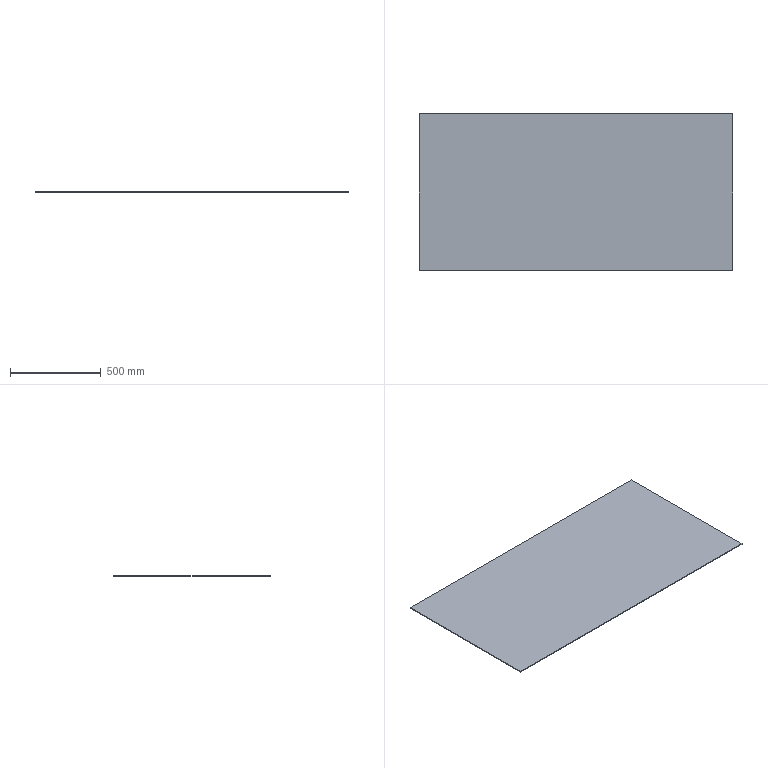Part | STEP file | 粉仓楼梯通道花纹Plate | 1 solid | 6 faces | box 1721 x 860 x 4 mm | volume 5920240 mm3 | plane 6
STEP:
#1=CARTESIAN_POINT('',(0.,0.,0.));
#2=DIRECTION('',(0.,0.,1.));
#3=DIRECTION('',(1.,0.,0.));
#4=AXIS2_PLACEMENT_3D('',#1,#2,#3);
#5=CARTESIAN_POINT('',(1588.,-50.,0.));
#6=VERTEX_POINT('',#5);
#7=CARTESIAN_POINT('',(1588.,810.,0.));
#8=VERTEX_POINT('',#7);
#9=CARTESIAN_POINT('',(1588.,810.,0.));
#10=DIRECTION('',(0.,1.,0.));
#11=VECTOR('',#10,1.);
#12=LINE('',#9,#11);
#13=CARTESIAN_POINT('',(1588.,810.,4.));
#14=DIRECTION('',(-1.,0.,0.));
#15=DIRECTION('',(0.,-1.,0.));
#16=AXIS2_PLACEMENT_3D('',#13,#14,#15);
#17=PLANE('',#16);
#18=CARTESIAN_POINT('',(0.,-4.));
#19=DIRECTION('',(-1.,0.));
#20=VECTOR('',#19,1.);
#21=LINE('',#18,#20);
#22=(GEOMETRIC_REPRESENTATION_CONTEXT(2)PARAMETRIC_REPRESENTATION_CONTEXT()REPRESENTATION_CONTEXT('',''));
#23=DEFINITIONAL_REPRESENTATION('',(#21),#22);
#24=PCURVE('',#17,#23);
#25=CARTESIAN_POINT('',(0.,0.,0.));
#26=DIRECTION('',(0.,0.,1.));
#27=DIRECTION('',(1.,0.,0.));
#28=AXIS2_PLACEMENT_3D('',#25,#26,#27);
#29=PLANE('',#28);
#30=CARTESIAN_POINT('',(1588.,810.));
#31=DIRECTION('',(0.,1.));
#32=VECTOR('',#31,1.);
#33=LINE('',#30,#32);
#34=(GEOMETRIC_REPRESENTATION_CONTEXT(2)PARAMETRIC_REPRESENTATION_CONTEXT()REPRESENTATION_CONTEXT('',''));
#35=DEFINITIONAL_REPRESENTATION('',(#33),#34);
#36=PCURVE('',#29,#35);
#37=SURFACE_CURVE('',#12,(#24,#36),.PCURVE_S1.);
#38=EDGE_CURVE('',#6,#8,#37,.T.);
#39=ORIENTED_EDGE('',*,*,#38,.T.);
#40=CARTESIAN_POINT('',(1588.,810.,4.));
#41=VERTEX_POINT('',#40);
#42=CARTESIAN_POINT('',(1588.,810.,4.));
#43=DIRECTION('',(0.,0.,-1.));
#44=VECTOR('',#43,1.);
#45=LINE('',#42,#44);
#46=CARTESIAN_POINT('',(0.,0.));
#47=DIRECTION('',(0.,-1.));
#48=VECTOR('',#47,1.);
#49=LINE('',#46,#48);
#50=(GEOMETRIC_REPRESENTATION_CONTEXT(2)PARAMETRIC_REPRESENTATION_CONTEXT()REPRESENTATION_CONTEXT('',''));
#51=DEFINITIONAL_REPRESENTATION('',(#49),#50);
#52=PCURVE('',#17,#51);
#53=CARTESIAN_POINT('',(-133.,810.,4.));
#54=DIRECTION('',(0.,-1.,0.));
#55=DIRECTION('',(1.,0.,0.));
#56=AXIS2_PLACEMENT_3D('',#53,#54,#55);
#57=PLANE('',#56);
#58=CARTESIAN_POINT('',(1721.,0.));
#59=DIRECTION('',(0.,-1.));
#60=VECTOR('',#59,1.);
#61=LINE('',#58,#60);
#62=(GEOMETRIC_REPRESENTATION_CONTEXT(2)PARAMETRIC_REPRESENTATION_CONTEXT()REPRESENTATION_CONTEXT('',''));
#63=DEFINITIONAL_REPRESENTATION('',(#61),#62);
#64=PCURVE('',#57,#63);
#65=SURFACE_CURVE('',#45,(#52,#64),.PCURVE_S1.);
#66=EDGE_CURVE('',#41,#8,#65,.T.);
#67=ORIENTED_EDGE('',*,*,#66,.F.);
#68=CARTESIAN_POINT('',(1588.,-50.,4.));
#69=VERTEX_POINT('',#68);
#70=CARTESIAN_POINT('',(1588.,810.,4.));
#71=DIRECTION('',(0.,1.,0.));
#72=VECTOR('',#71,1.);
#73=LINE('',#70,#72);
#74=CARTESIAN_POINT('',(0.,0.));
#75=DIRECTION('',(-1.,0.));
#76=VECTOR('',#75,1.);
#77=LINE('',#74,#76);
#78=(GEOMETRIC_REPRESENTATION_CONTEXT(2)PARAMETRIC_REPRESENTATION_CONTEXT()REPRESENTATION_CONTEXT('',''));
#79=DEFINITIONAL_REPRESENTATION('',(#77),#78);
#80=PCURVE('',#17,#79);
#81=CARTESIAN_POINT('',(0.,0.,4.));
#82=DIRECTION('',(0.,0.,1.));
#83=DIRECTION('',(1.,0.,0.));
#84=AXIS2_PLACEMENT_3D('',#81,#82,#83);
#85=PLANE('',#84);
#86=CARTESIAN_POINT('',(1588.,810.));
#87=DIRECTION('',(0.,1.));
#88=VECTOR('',#87,1.);
#89=LINE('',#86,#88);
#90=(GEOMETRIC_REPRESENTATION_CONTEXT(2)PARAMETRIC_REPRESENTATION_CONTEXT()REPRESENTATION_CONTEXT('',''));
#91=DEFINITIONAL_REPRESENTATION('',(#89),#90);
#92=PCURVE('',#85,#91);
#93=SURFACE_CURVE('',#73,(#80,#92),.PCURVE_S1.);
#94=EDGE_CURVE('',#69,#41,#93,.T.);
#95=ORIENTED_EDGE('',*,*,#94,.F.);
#96=CARTESIAN_POINT('',(1588.,-50.,4.));
#97=DIRECTION('',(0.,0.,-1.));
#98=VECTOR('',#97,1.);
#99=LINE('',#96,#98);
#100=CARTESIAN_POINT('',(860.,0.));
#101=DIRECTION('',(0.,-1.));
#102=VECTOR('',#101,1.);
#103=LINE('',#100,#102);
#104=(GEOMETRIC_REPRESENTATION_CONTEXT(2)PARAMETRIC_REPRESENTATION_CONTEXT()REPRESENTATION_CONTEXT('',''));
#105=DEFINITIONAL_REPRESENTATION('',(#103),#104);
#106=PCURVE('',#17,#105);
#107=CARTESIAN_POINT('',(-133.,-50.,4.));
#108=DIRECTION('',(0.,1.,0.));
#109=DIRECTION('',(-1.,0.,0.));
#110=AXIS2_PLACEMENT_3D('',#107,#108,#109);
#111=PLANE('',#110);
#112=CARTESIAN_POINT('',(-1721.,0.));
#113=DIRECTION('',(0.,-1.));
#114=VECTOR('',#113,1.);
#115=LINE('',#112,#114);
#116=(GEOMETRIC_REPRESENTATION_CONTEXT(2)PARAMETRIC_REPRESENTATION_CONTEXT()REPRESENTATION_CONTEXT('',''));
#117=DEFINITIONAL_REPRESENTATION('',(#115),#116);
#118=PCURVE('',#111,#117);
#119=SURFACE_CURVE('',#99,(#106,#118),.PCURVE_S1.);
#120=EDGE_CURVE('',#69,#6,#119,.T.);
#121=ORIENTED_EDGE('',*,*,#120,.T.);
#122=EDGE_LOOP('',(#39,#67,#95,#121));
#123=FACE_BOUND('',#122,.T.);
#124=ADVANCED_FACE('',(#123),#17,.F.);
#125=CARTESIAN_POINT('',(-133.,810.,0.));
#126=VERTEX_POINT('',#125);
#127=CARTESIAN_POINT('',(-133.,810.,0.));
#128=DIRECTION('',(-1.,0.,0.));
#129=VECTOR('',#128,1.);
#130=LINE('',#127,#129);
#131=CARTESIAN_POINT('',(0.,-4.));
#132=DIRECTION('',(-1.,0.));
#133=VECTOR('',#132,1.);
#134=LINE('',#131,#133);
#135=(GEOMETRIC_REPRESENTATION_CONTEXT(2)PARAMETRIC_REPRESENTATION_CONTEXT()REPRESENTATION_CONTEXT('',''));
#136=DEFINITIONAL_REPRESENTATION('',(#134),#135);
#137=PCURVE('',#57,#136);
#138=CARTESIAN_POINT('',(-133.,810.));
#139=DIRECTION('',(-1.,0.));
#140=VECTOR('',#139,1.);
#141=LINE('',#138,#140);
#142=(GEOMETRIC_REPRESENTATION_CONTEXT(2)PARAMETRIC_REPRESENTATION_CONTEXT()REPRESENTATION_CONTEXT('',''));
#143=DEFINITIONAL_REPRESENTATION('',(#141),#142);
#144=PCURVE('',#29,#143);
#145=SURFACE_CURVE('',#130,(#137,#144),.PCURVE_S1.);
#146=EDGE_CURVE('',#8,#126,#145,.T.);
#147=ORIENTED_EDGE('',*,*,#146,.T.);
#148=CARTESIAN_POINT('',(-133.,810.,4.));
#149=VERTEX_POINT('',#148);
#150=CARTESIAN_POINT('',(-133.,810.,4.));
#151=DIRECTION('',(0.,0.,-1.));
#152=VECTOR('',#151,1.);
#153=LINE('',#150,#152);
#154=CARTESIAN_POINT('',(0.,0.));
#155=DIRECTION('',(0.,-1.));
#156=VECTOR('',#155,1.);
#157=LINE('',#154,#156);
#158=(GEOMETRIC_REPRESENTATION_CONTEXT(2)PARAMETRIC_REPRESENTATION_CONTEXT()REPRESENTATION_CONTEXT('',''));
#159=DEFINITIONAL_REPRESENTATION('',(#157),#158);
#160=PCURVE('',#57,#159);
#161=CARTESIAN_POINT('',(-133.,810.,4.));
#162=DIRECTION('',(1.,0.,0.));
#163=DIRECTION('',(0.,1.,0.));
#164=AXIS2_PLACEMENT_3D('',#161,#162,#163);
#165=PLANE('',#164);
#166=CARTESIAN_POINT('',(0.,0.));
#167=DIRECTION('',(0.,-1.));
#168=VECTOR('',#167,1.);
#169=LINE('',#166,#168);
#170=(GEOMETRIC_REPRESENTATION_CONTEXT(2)PARAMETRIC_REPRESENTATION_CONTEXT()REPRESENTATION_CONTEXT('',''));
#171=DEFINITIONAL_REPRESENTATION('',(#169),#170);
#172=PCURVE('',#165,#171);
#173=SURFACE_CURVE('',#153,(#160,#172),.PCURVE_S1.);
#174=EDGE_CURVE('',#149,#126,#173,.T.);
#175=ORIENTED_EDGE('',*,*,#174,.F.);
#176=CARTESIAN_POINT('',(-133.,810.,4.));
#177=DIRECTION('',(-1.,0.,0.));
#178=VECTOR('',#177,1.);
#179=LINE('',#176,#178);
#180=CARTESIAN_POINT('',(0.,0.));
#181=DIRECTION('',(-1.,0.));
#182=VECTOR('',#181,1.);
#183=LINE('',#180,#182);
#184=(GEOMETRIC_REPRESENTATION_CONTEXT(2)PARAMETRIC_REPRESENTATION_CONTEXT()REPRESENTATION_CONTEXT('',''));
#185=DEFINITIONAL_REPRESENTATION('',(#183),#184);
#186=PCURVE('',#57,#185);
#187=CARTESIAN_POINT('',(-133.,810.));
#188=DIRECTION('',(-1.,0.));
#189=VECTOR('',#188,1.);
#190=LINE('',#187,#189);
#191=(GEOMETRIC_REPRESENTATION_CONTEXT(2)PARAMETRIC_REPRESENTATION_CONTEXT()REPRESENTATION_CONTEXT('',''));
#192=DEFINITIONAL_REPRESENTATION('',(#190),#191);
#193=PCURVE('',#85,#192);
#194=SURFACE_CURVE('',#179,(#186,#193),.PCURVE_S1.);
#195=EDGE_CURVE('',#41,#149,#194,.T.);
#196=ORIENTED_EDGE('',*,*,#195,.F.);
#197=ORIENTED_EDGE('',*,*,#66,.T.);
#198=EDGE_LOOP('',(#147,#175,#196,#197));
#199=FACE_BOUND('',#198,.T.);
#200=ADVANCED_FACE('',(#199),#57,.F.);
#201=CARTESIAN_POINT('',(-133.,-50.,0.));
#202=VERTEX_POINT('',#201);
#203=CARTESIAN_POINT('',(-133.,810.,0.));
#204=DIRECTION('',(0.,-1.,0.));
#205=VECTOR('',#204,1.);
#206=LINE('',#203,#205);
#207=CARTESIAN_POINT('',(0.,-4.));
#208=DIRECTION('',(-1.,0.));
#209=VECTOR('',#208,1.);
#210=LINE('',#207,#209);
#211=(GEOMETRIC_REPRESENTATION_CONTEXT(2)PARAMETRIC_REPRESENTATION_CONTEXT()REPRESENTATION_CONTEXT('',''));
#212=DEFINITIONAL_REPRESENTATION('',(#210),#211);
#213=PCURVE('',#165,#212);
#214=CARTESIAN_POINT('',(-133.,810.));
#215=DIRECTION('',(0.,-1.));
#216=VECTOR('',#215,1.);
#217=LINE('',#214,#216);
#218=(GEOMETRIC_REPRESENTATION_CONTEXT(2)PARAMETRIC_REPRESENTATION_CONTEXT()REPRESENTATION_CONTEXT('',''));
#219=DEFINITIONAL_REPRESENTATION('',(#217),#218);
#220=PCURVE('',#29,#219);
#221=SURFACE_CURVE('',#206,(#213,#220),.PCURVE_S1.);
#222=EDGE_CURVE('',#126,#202,#221,.T.);
#223=ORIENTED_EDGE('',*,*,#222,.T.);
#224=CARTESIAN_POINT('',(-133.,-50.,4.));
#225=VERTEX_POINT('',#224);
#226=CARTESIAN_POINT('',(-133.,-50.,4.));
#227=DIRECTION('',(0.,0.,-1.));
#228=VECTOR('',#227,1.);
#229=LINE('',#226,#228);
#230=CARTESIAN_POINT('',(-860.,0.));
#231=DIRECTION('',(0.,-1.));
#232=VECTOR('',#231,1.);
#233=LINE('',#230,#232);
#234=(GEOMETRIC_REPRESENTATION_CONTEXT(2)PARAMETRIC_REPRESENTATION_CONTEXT()REPRESENTATION_CONTEXT('',''));
#235=DEFINITIONAL_REPRESENTATION('',(#233),#234);
#236=PCURVE('',#165,#235);
#237=CARTESIAN_POINT('',(0.,0.));
#238=DIRECTION('',(0.,-1.));
#239=VECTOR('',#238,1.);
#240=LINE('',#237,#239);
#241=(GEOMETRIC_REPRESENTATION_CONTEXT(2)PARAMETRIC_REPRESENTATION_CONTEXT()REPRESENTATION_CONTEXT('',''));
#242=DEFINITIONAL_REPRESENTATION('',(#240),#241);
#243=PCURVE('',#111,#242);
#244=SURFACE_CURVE('',#229,(#236,#243),.PCURVE_S1.);
#245=EDGE_CURVE('',#225,#202,#244,.T.);
#246=ORIENTED_EDGE('',*,*,#245,.F.);
#247=CARTESIAN_POINT('',(-133.,810.,4.));
#248=DIRECTION('',(0.,-1.,0.));
#249=VECTOR('',#248,1.);
#250=LINE('',#247,#249);
#251=CARTESIAN_POINT('',(0.,0.));
#252=DIRECTION('',(-1.,0.));
#253=VECTOR('',#252,1.);
#254=LINE('',#251,#253);
#255=(GEOMETRIC_REPRESENTATION_CONTEXT(2)PARAMETRIC_REPRESENTATION_CONTEXT()REPRESENTATION_CONTEXT('',''));
#256=DEFINITIONAL_REPRESENTATION('',(#254),#255);
#257=PCURVE('',#165,#256);
#258=CARTESIAN_POINT('',(-133.,810.));
#259=DIRECTION('',(0.,-1.));
#260=VECTOR('',#259,1.);
#261=LINE('',#258,#260);
#262=(GEOMETRIC_REPRESENTATION_CONTEXT(2)PARAMETRIC_REPRESENTATION_CONTEXT()REPRESENTATION_CONTEXT('',''));
#263=DEFINITIONAL_REPRESENTATION('',(#261),#262);
#264=PCURVE('',#85,#263);
#265=SURFACE_CURVE('',#250,(#257,#264),.PCURVE_S1.);
#266=EDGE_CURVE('',#149,#225,#265,.T.);
#267=ORIENTED_EDGE('',*,*,#266,.F.);
#268=ORIENTED_EDGE('',*,*,#174,.T.);
#269=EDGE_LOOP('',(#223,#246,#267,#268));
#270=FACE_BOUND('',#269,.T.);
#271=ADVANCED_FACE('',(#270),#165,.F.);
#272=CARTESIAN_POINT('',(-133.,-50.,0.));
#273=DIRECTION('',(1.,0.,0.));
#274=VECTOR('',#273,1.);
#275=LINE('',#272,#274);
#276=CARTESIAN_POINT('',(0.,-4.));
#277=DIRECTION('',(-1.,0.));
#278=VECTOR('',#277,1.);
#279=LINE('',#276,#278);
#280=(GEOMETRIC_REPRESENTATION_CONTEXT(2)PARAMETRIC_REPRESENTATION_CONTEXT()REPRESENTATION_CONTEXT('',''));
#281=DEFINITIONAL_REPRESENTATION('',(#279),#280);
#282=PCURVE('',#111,#281);
#283=CARTESIAN_POINT('',(-133.,-50.));
#284=DIRECTION('',(1.,0.));
#285=VECTOR('',#284,1.);
#286=LINE('',#283,#285);
#287=(GEOMETRIC_REPRESENTATION_CONTEXT(2)PARAMETRIC_REPRESENTATION_CONTEXT()REPRESENTATION_CONTEXT('',''));
#288=DEFINITIONAL_REPRESENTATION('',(#286),#287);
#289=PCURVE('',#29,#288);
#290=SURFACE_CURVE('',#275,(#282,#289),.PCURVE_S1.);
#291=EDGE_CURVE('',#202,#6,#290,.T.);
#292=ORIENTED_EDGE('',*,*,#291,.T.);
#293=ORIENTED_EDGE('',*,*,#120,.F.);
#294=CARTESIAN_POINT('',(-133.,-50.,4.));
#295=DIRECTION('',(1.,0.,0.));
#296=VECTOR('',#295,1.);
#297=LINE('',#294,#296);
#298=CARTESIAN_POINT('',(0.,0.));
#299=DIRECTION('',(-1.,0.));
#300=VECTOR('',#299,1.);
#301=LINE('',#298,#300);
#302=(GEOMETRIC_REPRESENTATION_CONTEXT(2)PARAMETRIC_REPRESENTATION_CONTEXT()REPRESENTATION_CONTEXT('',''));
#303=DEFINITIONAL_REPRESENTATION('',(#301),#302);
#304=PCURVE('',#111,#303);
#305=CARTESIAN_POINT('',(-133.,-50.));
#306=DIRECTION('',(1.,0.));
#307=VECTOR('',#306,1.);
#308=LINE('',#305,#307);
#309=(GEOMETRIC_REPRESENTATION_CONTEXT(2)PARAMETRIC_REPRESENTATION_CONTEXT()REPRESENTATION_CONTEXT('',''));
#310=DEFINITIONAL_REPRESENTATION('',(#308),#309);
#311=PCURVE('',#85,#310);
#312=SURFACE_CURVE('',#297,(#304,#311),.PCURVE_S1.);
#313=EDGE_CURVE('',#225,#69,#312,.T.);
#314=ORIENTED_EDGE('',*,*,#313,.F.);
#315=ORIENTED_EDGE('',*,*,#245,.T.);
#316=EDGE_LOOP('',(#292,#293,#314,#315));
#317=FACE_BOUND('',#316,.T.);
#318=ADVANCED_FACE('',(#317),#111,.F.);
#319=ORIENTED_EDGE('',*,*,#94,.T.);
#320=ORIENTED_EDGE('',*,*,#195,.T.);
#321=ORIENTED_EDGE('',*,*,#266,.T.);
#322=ORIENTED_EDGE('',*,*,#313,.T.);
#323=EDGE_LOOP('',(#319,#320,#321,#322));
#324=FACE_BOUND('',#323,.T.);
#325=ADVANCED_FACE('',(#324),#85,.T.);
#326=ORIENTED_EDGE('',*,*,#38,.F.);
#327=ORIENTED_EDGE('',*,*,#291,.F.);
#328=ORIENTED_EDGE('',*,*,#222,.F.);
#329=ORIENTED_EDGE('',*,*,#146,.F.);
#330=EDGE_LOOP('',(#326,#327,#328,#329));
#331=FACE_BOUND('',#330,.T.);
#332=ADVANCED_FACE('',(#331),#29,.F.);
#333=CLOSED_SHELL('',(#124,#200,#271,#318,#325,#332));
#334=MANIFOLD_SOLID_BREP('',#333);
#335=(LENGTH_UNIT()NAMED_UNIT(*)SI_UNIT(.MILLI.,.METRE.));
#336=UNCERTAINTY_MEASURE_WITH_UNIT(LENGTH_MEASURE(0.0000001),#335,'','');
#337=(NAMED_UNIT(*)PLANE_ANGLE_UNIT()SI_UNIT($,.RADIAN.));
#338=(NAMED_UNIT(*)SI_UNIT($,.STERADIAN.)SOLID_ANGLE_UNIT());
#339=(GEOMETRIC_REPRESENTATION_CONTEXT(3)GLOBAL_UNCERTAINTY_ASSIGNED_CONTEXT((#336))GLOBAL_UNIT_ASSIGNED_CONTEXT((#335,#337,#338))REPRESENTATION_CONTEXT('',''));
#340=ADVANCED_BREP_SHAPE_REPRESENTATION('',(#4,#334),#339);